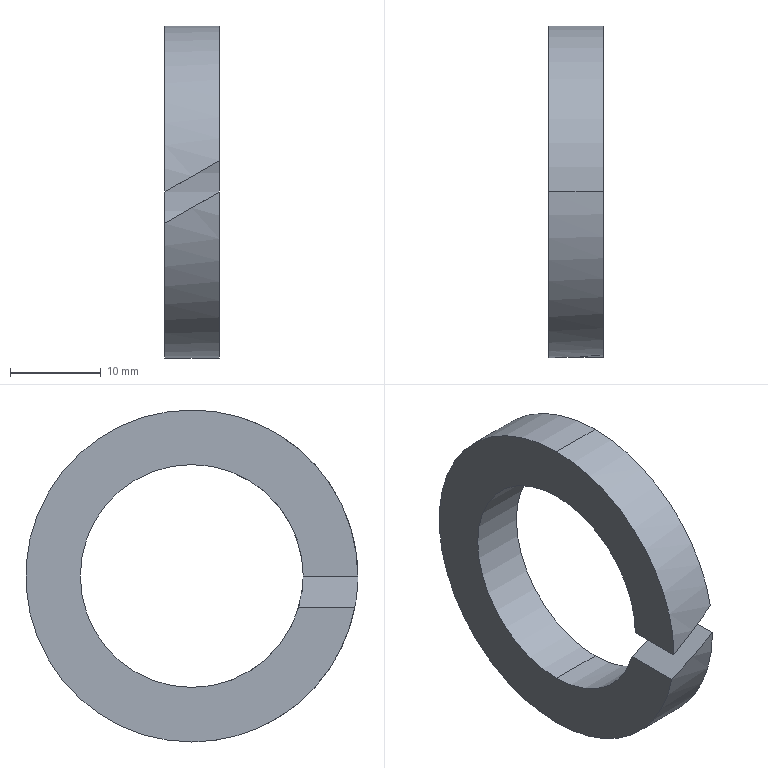Part | SolidWorks | features BaseBody 1 | 1 solid | 10 faces | box 6 x 36.5 x 36.5 mm | volume 3324 mm3 | cylinder 6 | plane 4 | commonest cylinder face diameters 24.5 x3 36.5 x3
STEP:
#1=CARTESIAN_POINT('',(-43.,-12.25,0.));
#2=VERTEX_POINT('',#1);
#3=CARTESIAN_POINT('',(-43.,0.,-12.25));
#4=VERTEX_POINT('',#3);
#5=CARTESIAN_POINT('',(-43.,0.,0.));
#6=DIRECTION('',(1.,0.,0.));
#7=DIRECTION('',(0.,0.,1.));
#8=AXIS2_PLACEMENT_3D('',#5,#6,#7);
#9=CIRCLE('',#8,12.25);
#10=EDGE_CURVE('',#2,#4,#9,.T.);
#11=ORIENTED_EDGE('',*,*,#10,.T.);
#12=CARTESIAN_POINT('',(-49.,0.,-12.25));
#13=VERTEX_POINT('',#12);
#14=CARTESIAN_POINT('',(-43.,0.,-12.25));
#15=DIRECTION('',(-1.,0.,0.));
#16=VECTOR('',#15,1000.);
#17=LINE('',#14,#16);
#18=EDGE_CURVE('',#4,#13,#17,.T.);
#19=ORIENTED_EDGE('',*,*,#18,.T.);
#20=CARTESIAN_POINT('',(-49.,-11.75,-3.464));
#21=VERTEX_POINT('',#20);
#22=CARTESIAN_POINT('',(-49.,0.,0.));
#23=DIRECTION('',(1.,0.,0.));
#24=DIRECTION('',(0.,0.,-1.));
#25=AXIS2_PLACEMENT_3D('',#22,#23,#24);
#26=CIRCLE('',#25,12.25);
#27=EDGE_CURVE('',#21,#13,#26,.T.);
#28=ORIENTED_EDGE('',*,*,#27,.F.);
#29=CARTESIAN_POINT('',(-49.,-11.75,-3.464));
#30=CARTESIAN_POINT('',(-47.048,-12.082,-2.337));
#31=CARTESIAN_POINT('',(-45.035,-12.25,-1.175));
#32=CARTESIAN_POINT('',(-43.,-12.25,0.));
#33=(BOUNDED_CURVE()B_SPLINE_CURVE(3,(#29,#30,#31,#32),.UNSPECIFIED.,.F.,.F.)B_SPLINE_CURVE_WITH_KNOTS((4,4),(1.284,1.571),.UNSPECIFIED.)CURVE()GEOMETRIC_REPRESENTATION_ITEM()RATIONAL_B_SPLINE_CURVE((1.,0.9932,0.9932,1.))REPRESENTATION_ITEM(''));
#34=EDGE_CURVE('',#21,#2,#33,.T.);
#35=ORIENTED_EDGE('',*,*,#34,.T.);
#36=EDGE_LOOP('',(#11,#19,#28,#35));
#37=FACE_OUTER_BOUND('',#36,.T.);
#38=CARTESIAN_POINT('',(-43.,0.,0.));
#39=DIRECTION('',(-1.,0.,0.));
#40=DIRECTION('',(0.,0.,1.));
#41=AXIS2_PLACEMENT_3D('',#38,#39,#40);
#42=CYLINDRICAL_SURFACE('',#41,12.25);
#43=ADVANCED_FACE('',(#37),#42,.F.);
#44=ORIENTED_EDGE('',*,*,#18,.F.);
#45=CARTESIAN_POINT('',(-43.,0.,12.25));
#46=VERTEX_POINT('',#45);
#47=CARTESIAN_POINT('',(-43.,0.,0.));
#48=DIRECTION('',(1.,0.,0.));
#49=DIRECTION('',(0.,0.,1.));
#50=AXIS2_PLACEMENT_3D('',#47,#48,#49);
#51=CIRCLE('',#50,12.25);
#52=EDGE_CURVE('',#4,#46,#51,.T.);
#53=ORIENTED_EDGE('',*,*,#52,.T.);
#54=CARTESIAN_POINT('',(-49.,0.,12.25));
#55=VERTEX_POINT('',#54);
#56=CARTESIAN_POINT('',(-43.,0.,12.25));
#57=DIRECTION('',(-1.,0.,0.));
#58=VECTOR('',#57,1000.);
#59=LINE('',#56,#58);
#60=EDGE_CURVE('',#46,#55,#59,.T.);
#61=ORIENTED_EDGE('',*,*,#60,.T.);
#62=CARTESIAN_POINT('',(-49.,0.,0.));
#63=DIRECTION('',(1.,0.,0.));
#64=DIRECTION('',(0.,0.,-1.));
#65=AXIS2_PLACEMENT_3D('',#62,#63,#64);
#66=CIRCLE('',#65,12.25);
#67=EDGE_CURVE('',#13,#55,#66,.T.);
#68=ORIENTED_EDGE('',*,*,#67,.F.);
#69=EDGE_LOOP('',(#44,#53,#61,#68));
#70=FACE_OUTER_BOUND('',#69,.T.);
#71=CARTESIAN_POINT('',(-43.,0.,0.));
#72=DIRECTION('',(-1.,0.,0.));
#73=DIRECTION('',(0.,0.,1.));
#74=AXIS2_PLACEMENT_3D('',#71,#72,#73);
#75=CYLINDRICAL_SURFACE('',#74,12.25);
#76=ADVANCED_FACE('',(#70),#75,.F.);
#77=CARTESIAN_POINT('',(-43.,0.,-18.25));
#78=VERTEX_POINT('',#77);
#79=CARTESIAN_POINT('',(-43.,0.,18.25));
#80=VERTEX_POINT('',#79);
#81=CARTESIAN_POINT('',(-43.,0.,0.));
#82=DIRECTION('',(1.,0.,0.));
#83=DIRECTION('',(0.,0.,1.));
#84=AXIS2_PLACEMENT_3D('',#81,#82,#83);
#85=CIRCLE('',#84,18.25);
#86=EDGE_CURVE('',#78,#80,#85,.T.);
#87=ORIENTED_EDGE('',*,*,#86,.F.);
#88=CARTESIAN_POINT('',(-49.,0.,-18.25));
#89=VERTEX_POINT('',#88);
#90=CARTESIAN_POINT('',(-43.,0.,-18.25));
#91=DIRECTION('',(-1.,0.,0.));
#92=VECTOR('',#91,1000.);
#93=LINE('',#90,#92);
#94=EDGE_CURVE('',#78,#89,#93,.T.);
#95=ORIENTED_EDGE('',*,*,#94,.T.);
#96=CARTESIAN_POINT('',(-49.,0.,18.25));
#97=VERTEX_POINT('',#96);
#98=CARTESIAN_POINT('',(-49.,0.,0.));
#99=DIRECTION('',(1.,0.,0.));
#100=DIRECTION('',(0.,0.,-1.));
#101=AXIS2_PLACEMENT_3D('',#98,#99,#100);
#102=CIRCLE('',#101,18.25);
#103=EDGE_CURVE('',#89,#97,#102,.T.);
#104=ORIENTED_EDGE('',*,*,#103,.T.);
#105=CARTESIAN_POINT('',(-43.,0.,18.25));
#106=DIRECTION('',(-1.,0.,0.));
#107=VECTOR('',#106,1000.);
#108=LINE('',#105,#107);
#109=EDGE_CURVE('',#80,#97,#108,.T.);
#110=ORIENTED_EDGE('',*,*,#109,.F.);
#111=EDGE_LOOP('',(#87,#95,#104,#110));
#112=FACE_OUTER_BOUND('',#111,.T.);
#113=CARTESIAN_POINT('',(-43.,0.,0.));
#114=DIRECTION('',(-1.,0.,0.));
#115=DIRECTION('',(0.,0.,1.));
#116=AXIS2_PLACEMENT_3D('',#113,#114,#115);
#117=CYLINDRICAL_SURFACE('',#116,18.25);
#118=ADVANCED_FACE('',(#112),#117,.T.);
#119=CARTESIAN_POINT('',(-43.,-17.918,3.464));
#120=VERTEX_POINT('',#119);
#121=CARTESIAN_POINT('',(-43.,0.,0.));
#122=DIRECTION('',(1.,0.,0.));
#123=DIRECTION('',(0.,0.,1.));
#124=AXIS2_PLACEMENT_3D('',#121,#122,#123);
#125=CIRCLE('',#124,18.25);
#126=EDGE_CURVE('',#80,#120,#125,.T.);
#127=ORIENTED_EDGE('',*,*,#126,.F.);
#128=ORIENTED_EDGE('',*,*,#109,.T.);
#129=CARTESIAN_POINT('',(-49.,-18.25,0.));
#130=VERTEX_POINT('',#129);
#131=CARTESIAN_POINT('',(-49.,0.,0.));
#132=DIRECTION('',(1.,0.,0.));
#133=DIRECTION('',(0.,0.,-1.));
#134=AXIS2_PLACEMENT_3D('',#131,#132,#133);
#135=CIRCLE('',#134,18.25);
#136=EDGE_CURVE('',#97,#130,#135,.T.);
#137=ORIENTED_EDGE('',*,*,#136,.T.);
#138=CARTESIAN_POINT('',(-43.,-17.918,3.464));
#139=CARTESIAN_POINT('',(-44.979,-18.139,2.322));
#140=CARTESIAN_POINT('',(-46.985,-18.25,1.164));
#141=CARTESIAN_POINT('',(-49.,-18.25,0.));
#142=(BOUNDED_CURVE()B_SPLINE_CURVE(3,(#138,#139,#140,#141),.UNSPECIFIED.,.F.,.T.)B_SPLINE_CURVE_WITH_KNOTS((4,4),(4.521,4.712),.UNSPECIFIED.)CURVE()GEOMETRIC_REPRESENTATION_ITEM()RATIONAL_B_SPLINE_CURVE((1.,0.997,0.997,1.))REPRESENTATION_ITEM(''));
#143=EDGE_CURVE('',#120,#130,#142,.T.);
#144=ORIENTED_EDGE('',*,*,#143,.F.);
#145=EDGE_LOOP('',(#127,#128,#137,#144));
#146=FACE_OUTER_BOUND('',#145,.T.);
#147=CARTESIAN_POINT('',(-43.,0.,0.));
#148=DIRECTION('',(-1.,0.,0.));
#149=DIRECTION('',(0.,0.,1.));
#150=AXIS2_PLACEMENT_3D('',#147,#148,#149);
#151=CYLINDRICAL_SURFACE('',#150,18.25);
#152=ADVANCED_FACE('',(#146),#151,.T.);
#153=ORIENTED_EDGE('',*,*,#10,.F.);
#154=CARTESIAN_POINT('',(-43.,-18.25,0.));
#155=VERTEX_POINT('',#154);
#156=CARTESIAN_POINT('',(-43.,-18.251,0.));
#157=DIRECTION('',(0.,1.,0.));
#158=VECTOR('',#157,1000.);
#159=LINE('',#156,#158);
#160=EDGE_CURVE('',#155,#2,#159,.T.);
#161=ORIENTED_EDGE('',*,*,#160,.F.);
#162=CARTESIAN_POINT('',(-43.,0.,0.));
#163=DIRECTION('',(1.,0.,0.));
#164=DIRECTION('',(0.,0.,1.));
#165=AXIS2_PLACEMENT_3D('',#162,#163,#164);
#166=CIRCLE('',#165,18.25);
#167=EDGE_CURVE('',#155,#78,#166,.T.);
#168=ORIENTED_EDGE('',*,*,#167,.T.);
#169=ORIENTED_EDGE('',*,*,#86,.T.);
#170=ORIENTED_EDGE('',*,*,#126,.T.);
#171=CARTESIAN_POINT('',(-43.,-11.75,3.464));
#172=VERTEX_POINT('',#171);
#173=CARTESIAN_POINT('',(-43.,-18.251,3.464));
#174=DIRECTION('',(0.,1.,0.));
#175=VECTOR('',#174,1000.);
#176=LINE('',#173,#175);
#177=EDGE_CURVE('',#120,#172,#176,.T.);
#178=ORIENTED_EDGE('',*,*,#177,.T.);
#179=CARTESIAN_POINT('',(-43.,0.,0.));
#180=DIRECTION('',(1.,0.,0.));
#181=DIRECTION('',(0.,0.,1.));
#182=AXIS2_PLACEMENT_3D('',#179,#180,#181);
#183=CIRCLE('',#182,12.25);
#184=EDGE_CURVE('',#46,#172,#183,.T.);
#185=ORIENTED_EDGE('',*,*,#184,.F.);
#186=ORIENTED_EDGE('',*,*,#52,.F.);
#187=EDGE_LOOP('',(#153,#161,#168,#169,#170,#178,#185,#186));
#188=FACE_OUTER_BOUND('',#187,.T.);
#189=CARTESIAN_POINT('',(-43.,0.,0.));
#190=DIRECTION('',(-1.,0.,0.));
#191=DIRECTION('',(0.,0.,1.));
#192=AXIS2_PLACEMENT_3D('',#189,#190,#191);
#193=PLANE('',#192);
#194=ADVANCED_FACE('',(#188),#193,.F.);
#195=CARTESIAN_POINT('',(-49.,-17.918,-3.464));
#196=VERTEX_POINT('',#195);
#197=CARTESIAN_POINT('',(-49.,-18.251,-3.464));
#198=DIRECTION('',(0.,1.,0.));
#199=VECTOR('',#198,1000.);
#200=LINE('',#197,#199);
#201=EDGE_CURVE('',#196,#21,#200,.T.);
#202=ORIENTED_EDGE('',*,*,#201,.T.);
#203=ORIENTED_EDGE('',*,*,#27,.T.);
#204=ORIENTED_EDGE('',*,*,#67,.T.);
#205=CARTESIAN_POINT('',(-49.,-12.25,0.));
#206=VERTEX_POINT('',#205);
#207=CARTESIAN_POINT('',(-49.,0.,0.));
#208=DIRECTION('',(1.,0.,0.));
#209=DIRECTION('',(0.,0.,-1.));
#210=AXIS2_PLACEMENT_3D('',#207,#208,#209);
#211=CIRCLE('',#210,12.25);
#212=EDGE_CURVE('',#55,#206,#211,.T.);
#213=ORIENTED_EDGE('',*,*,#212,.T.);
#214=CARTESIAN_POINT('',(-49.,-18.251,0.));
#215=DIRECTION('',(0.,1.,0.));
#216=VECTOR('',#215,1000.);
#217=LINE('',#214,#216);
#218=EDGE_CURVE('',#130,#206,#217,.T.);
#219=ORIENTED_EDGE('',*,*,#218,.F.);
#220=ORIENTED_EDGE('',*,*,#136,.F.);
#221=ORIENTED_EDGE('',*,*,#103,.F.);
#222=CARTESIAN_POINT('',(-49.,0.,0.));
#223=DIRECTION('',(1.,0.,0.));
#224=DIRECTION('',(0.,0.,-1.));
#225=AXIS2_PLACEMENT_3D('',#222,#223,#224);
#226=CIRCLE('',#225,18.25);
#227=EDGE_CURVE('',#196,#89,#226,.T.);
#228=ORIENTED_EDGE('',*,*,#227,.F.);
#229=EDGE_LOOP('',(#202,#203,#204,#213,#219,#220,#221,#228));
#230=FACE_OUTER_BOUND('',#229,.T.);
#231=CARTESIAN_POINT('',(-49.,0.,0.));
#232=DIRECTION('',(-1.,0.,0.));
#233=DIRECTION('',(0.,0.,1.));
#234=AXIS2_PLACEMENT_3D('',#231,#232,#233);
#235=PLANE('',#234);
#236=ADVANCED_FACE('',(#230),#235,.T.);
#237=ORIENTED_EDGE('',*,*,#94,.F.);
#238=ORIENTED_EDGE('',*,*,#167,.F.);
#239=CARTESIAN_POINT('',(-49.,-17.918,-3.464));
#240=CARTESIAN_POINT('',(-47.021,-18.139,-2.322));
#241=CARTESIAN_POINT('',(-45.015,-18.25,-1.164));
#242=CARTESIAN_POINT('',(-43.,-18.25,0.));
#243=(BOUNDED_CURVE()B_SPLINE_CURVE(3,(#239,#240,#241,#242),.UNSPECIFIED.,.F.,.F.)B_SPLINE_CURVE_WITH_KNOTS((4,4),(1.38,1.571),.UNSPECIFIED.)CURVE()GEOMETRIC_REPRESENTATION_ITEM()RATIONAL_B_SPLINE_CURVE((1.,0.997,0.997,1.))REPRESENTATION_ITEM(''));
#244=EDGE_CURVE('',#196,#155,#243,.T.);
#245=ORIENTED_EDGE('',*,*,#244,.F.);
#246=ORIENTED_EDGE('',*,*,#227,.T.);
#247=EDGE_LOOP('',(#237,#238,#245,#246));
#248=FACE_OUTER_BOUND('',#247,.T.);
#249=CARTESIAN_POINT('',(-43.,0.,0.));
#250=DIRECTION('',(-1.,0.,0.));
#251=DIRECTION('',(0.,0.,1.));
#252=AXIS2_PLACEMENT_3D('',#249,#250,#251);
#253=CYLINDRICAL_SURFACE('',#252,18.25);
#254=ADVANCED_FACE('',(#248),#253,.T.);
#255=ORIENTED_EDGE('',*,*,#60,.F.);
#256=ORIENTED_EDGE('',*,*,#184,.T.);
#257=CARTESIAN_POINT('',(-43.,-11.75,3.464));
#258=CARTESIAN_POINT('',(-44.952,-12.082,2.337));
#259=CARTESIAN_POINT('',(-46.965,-12.25,1.175));
#260=CARTESIAN_POINT('',(-49.,-12.25,0.));
#261=(BOUNDED_CURVE()B_SPLINE_CURVE(3,(#257,#258,#259,#260),.UNSPECIFIED.,.F.,.F.)B_SPLINE_CURVE_WITH_KNOTS((4,4),(4.426,4.712),.UNSPECIFIED.)CURVE()GEOMETRIC_REPRESENTATION_ITEM()RATIONAL_B_SPLINE_CURVE((1.,0.9932,0.9932,1.))REPRESENTATION_ITEM(''));
#262=EDGE_CURVE('',#172,#206,#261,.T.);
#263=ORIENTED_EDGE('',*,*,#262,.T.);
#264=ORIENTED_EDGE('',*,*,#212,.F.);
#265=EDGE_LOOP('',(#255,#256,#263,#264));
#266=FACE_OUTER_BOUND('',#265,.T.);
#267=CARTESIAN_POINT('',(-43.,0.,0.));
#268=DIRECTION('',(-1.,0.,0.));
#269=DIRECTION('',(0.,0.,1.));
#270=AXIS2_PLACEMENT_3D('',#267,#268,#269);
#271=CYLINDRICAL_SURFACE('',#270,12.25);
#272=ADVANCED_FACE('',(#266),#271,.F.);
#273=ORIENTED_EDGE('',*,*,#143,.T.);
#274=ORIENTED_EDGE('',*,*,#218,.T.);
#275=ORIENTED_EDGE('',*,*,#262,.F.);
#276=ORIENTED_EDGE('',*,*,#177,.F.);
#277=EDGE_LOOP('',(#273,#274,#275,#276));
#278=FACE_OUTER_BOUND('',#277,.T.);
#279=CARTESIAN_POINT('',(-43.,-18.251,3.464));
#280=DIRECTION('',(-0.5,0.,0.866));
#281=DIRECTION('',(0.866,0.,0.5));
#282=AXIS2_PLACEMENT_3D('',#279,#280,#281);
#283=PLANE('',#282);
#284=ADVANCED_FACE('',(#278),#283,.F.);
#285=ORIENTED_EDGE('',*,*,#244,.T.);
#286=ORIENTED_EDGE('',*,*,#160,.T.);
#287=ORIENTED_EDGE('',*,*,#34,.F.);
#288=ORIENTED_EDGE('',*,*,#201,.F.);
#289=EDGE_LOOP('',(#285,#286,#287,#288));
#290=FACE_OUTER_BOUND('',#289,.T.);
#291=CARTESIAN_POINT('',(-49.,-18.251,-3.464));
#292=DIRECTION('',(0.5,0.,-0.866));
#293=DIRECTION('',(-0.866,0.,-0.5));
#294=AXIS2_PLACEMENT_3D('',#291,#292,#293);
#295=PLANE('',#294);
#296=ADVANCED_FACE('',(#290),#295,.F.);
#297=CLOSED_SHELL('',(#43,#76,#118,#152,#194,#236,#254,#272,#284,#296));
#298=MANIFOLD_SOLID_BREP('',#297);
#299=CARTESIAN_POINT('',(0.,0.,0.));
#300=DIRECTION('',(0.,0.,1.));
#301=DIRECTION('',(1.,0.,0.));
#302=AXIS2_PLACEMENT_3D('',#299,#300,#301);
#303=(LENGTH_UNIT()NAMED_UNIT(*)SI_UNIT(.MILLI.,.METRE.));
#304=UNCERTAINTY_MEASURE_WITH_UNIT(LENGTH_MEASURE(0.00001),#303,'','');
#305=(NAMED_UNIT(*)PLANE_ANGLE_UNIT()SI_UNIT($,.RADIAN.));
#306=(NAMED_UNIT(*)SI_UNIT($,.STERADIAN.)SOLID_ANGLE_UNIT());
#307=(GEOMETRIC_REPRESENTATION_CONTEXT(3)GLOBAL_UNCERTAINTY_ASSIGNED_CONTEXT((#304))GLOBAL_UNIT_ASSIGNED_CONTEXT((#303,#305,#306))REPRESENTATION_CONTEXT('',''));
#308=ADVANCED_BREP_SHAPE_REPRESENTATION('',(#298,#302),#307);